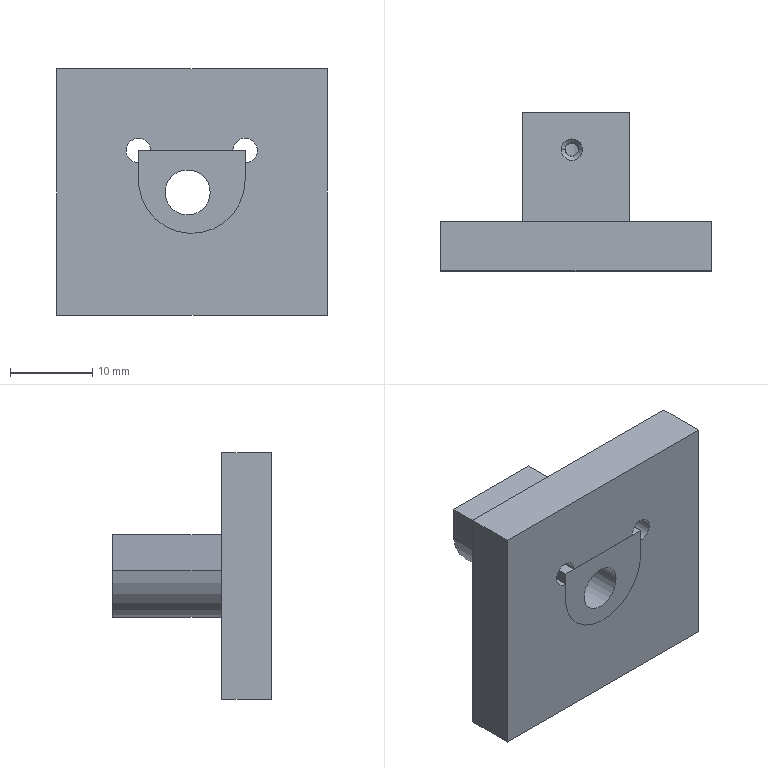NC program | NX | posted with a generic post | part box 32.951 x 19.3 x 30.1 mm
Whole program:
N10 G17 G21 G94 G90
(FLOOR_WALL_COPY_COPY , TOOL : D63)
N12 T01 M6
N14 G54
N16 G17 G0 G90 X44.6 Y0. B0. C0. S6500 M3
N18 G43 Z30. H1
N20 Z7.
N22 G94 G1 Z4. F1500.
N24 X41.6
N26 X-31.5
N28 X-34.5
N30 Z7.
N32 G0 Z30.
N34 X44.6
N36 Z6.
N38 G1 Z3.
N40 X41.6
N42 X-31.5
N44 X-34.5
N46 Z6.
N48 G0 Z30.
N50 X44.6
N52 Z5.
N54 G1 Z2.
N56 X41.6
N58 X-31.5
N60 X-34.5
N62 Z5.
N64 G0 Z30.
N66 X44.6
N68 Z4.
N70 G1 Z1.
N72 X41.6
N74 X-31.5
N76 X-34.5
N78 Z4.
N80 G0 Z30.
N82 X44.6
N84 Z3.
N86 G1 Z0.
N88 X41.6
N90 X-31.5
N92 X-34.5
N94 Z3.
N96 G0 Z30.
N98 M5
(PLANAR_MILL_COPY_COPY_COPY , TOOL : D6A45)
N100 T07 M6
N102 G54
N104 G17 G0 G90 X-1.257 Y-0.766 B0. C0. S9500 M3
N106 G43 Z30. H7
N108 Z0.5
N110 G94 G1 Z-1. F1250.
N112 G3 X-0.9 Y0. R1.
N114 G1 Y6.5
N116 G2 X0. Y7.4 R0.9
N118 G1 X3.6
N120 G2 X4.505 Y-7.345 R7.4
N122 G1 X4.405 Y-7.351
N124 X0.01 Y-7.4
N126 G2 X-0.9 Y-6.5 R0.9
N128 G1 Y0.
N130 G3 X-1.257 Y0.766 R1.
N132 G1 Z0.5
N134 G0 Z30.
N136 X3.607 Y0.266
N138 Z0.5
N140 G1 Z-1.
N142 G3 X3.25 Y-0.5 R1.
N144 X5.1 Y-2.35 R1.85
N146 X3.25 Y-0.5 R-1.85
N148 X3.607 Y-1.266 R1.
N150 G1 Z0.5
N152 G0 Z30.
N154 M5
N156 M2